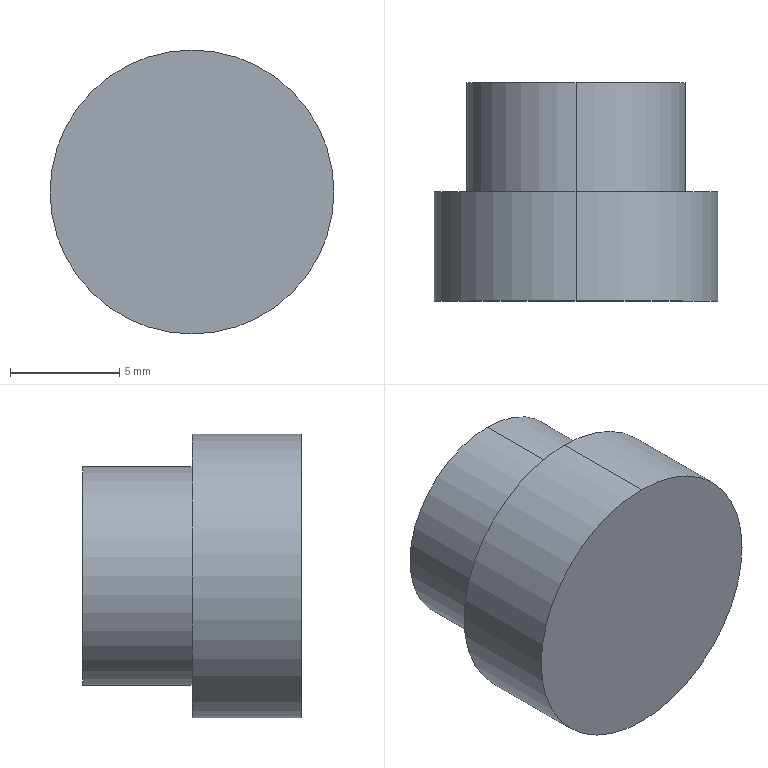Part | SolidWorks | features Revolution 1 | 1 solid | 10 faces | box 13 x 10 x 13 mm | volume 805.033 mm3 | cylinder 6 | plane 4 | commonest cylinder face diameters 8 x2 10 x2 13 x2
STEP:
#1=CARTESIAN_POINT('',(0.,10.,4.));
#2=VERTEX_POINT('',#1);
#3=CARTESIAN_POINT('',(0.,10.,-4.));
#4=VERTEX_POINT('',#3);
#5=CARTESIAN_POINT('',(0.,10.,0.));
#6=DIRECTION('',(0.,-1.,0.));
#7=DIRECTION('',(0.,0.,-1.));
#8=AXIS2_PLACEMENT_3D('',#5,#6,#7);
#9=CIRCLE('',#8,4.);
#10=EDGE_CURVE('',#2,#4,#9,.T.);
#11=ORIENTED_EDGE('',*,*,#10,.F.);
#12=CARTESIAN_POINT('',(0.,5.,4.));
#13=VERTEX_POINT('',#12);
#14=CARTESIAN_POINT('',(0.,0.,4.));
#15=DIRECTION('',(0.,-1.,0.));
#16=VECTOR('',#15,1000.);
#17=LINE('',#14,#16);
#18=EDGE_CURVE('',#2,#13,#17,.T.);
#19=ORIENTED_EDGE('',*,*,#18,.T.);
#20=CARTESIAN_POINT('',(0.,5.,-4.));
#21=VERTEX_POINT('',#20);
#22=CARTESIAN_POINT('',(0.,5.,0.));
#23=DIRECTION('',(0.,-1.,0.));
#24=DIRECTION('',(0.,0.,-1.));
#25=AXIS2_PLACEMENT_3D('',#22,#23,#24);
#26=CIRCLE('',#25,4.);
#27=EDGE_CURVE('',#13,#21,#26,.T.);
#28=ORIENTED_EDGE('',*,*,#27,.T.);
#29=CARTESIAN_POINT('',(0.,0.,-4.));
#30=DIRECTION('',(0.,-1.,0.));
#31=VECTOR('',#30,1000.);
#32=LINE('',#29,#31);
#33=EDGE_CURVE('',#4,#21,#32,.T.);
#34=ORIENTED_EDGE('',*,*,#33,.F.);
#35=EDGE_LOOP('',(#11,#19,#28,#34));
#36=FACE_OUTER_BOUND('',#35,.T.);
#37=CARTESIAN_POINT('',(0.,0.,0.));
#38=DIRECTION('',(0.,-1.,0.));
#39=DIRECTION('',(0.,0.,-1.));
#40=AXIS2_PLACEMENT_3D('',#37,#38,#39);
#41=CYLINDRICAL_SURFACE('',#40,4.);
#42=ADVANCED_FACE('',(#36),#41,.F.);
#43=CARTESIAN_POINT('',(0.,10.,-5.));
#44=VERTEX_POINT('',#43);
#45=CARTESIAN_POINT('',(0.,10.,5.));
#46=VERTEX_POINT('',#45);
#47=CARTESIAN_POINT('',(0.,10.,0.));
#48=DIRECTION('',(0.,-1.,0.));
#49=DIRECTION('',(0.,0.,-1.));
#50=AXIS2_PLACEMENT_3D('',#47,#48,#49);
#51=CIRCLE('',#50,5.);
#52=EDGE_CURVE('',#44,#46,#51,.T.);
#53=ORIENTED_EDGE('',*,*,#52,.T.);
#54=CARTESIAN_POINT('',(0.,5.,5.));
#55=VERTEX_POINT('',#54);
#56=CARTESIAN_POINT('',(0.,0.,5.));
#57=DIRECTION('',(0.,-1.,0.));
#58=VECTOR('',#57,1000.);
#59=LINE('',#56,#58);
#60=EDGE_CURVE('',#46,#55,#59,.T.);
#61=ORIENTED_EDGE('',*,*,#60,.T.);
#62=CARTESIAN_POINT('',(0.,5.,-5.));
#63=VERTEX_POINT('',#62);
#64=CARTESIAN_POINT('',(0.,5.,0.));
#65=DIRECTION('',(0.,-1.,0.));
#66=DIRECTION('',(0.,0.,-1.));
#67=AXIS2_PLACEMENT_3D('',#64,#65,#66);
#68=CIRCLE('',#67,5.);
#69=EDGE_CURVE('',#63,#55,#68,.T.);
#70=ORIENTED_EDGE('',*,*,#69,.F.);
#71=CARTESIAN_POINT('',(0.,0.,-5.));
#72=DIRECTION('',(0.,-1.,0.));
#73=VECTOR('',#72,1000.);
#74=LINE('',#71,#73);
#75=EDGE_CURVE('',#44,#63,#74,.T.);
#76=ORIENTED_EDGE('',*,*,#75,.F.);
#77=EDGE_LOOP('',(#53,#61,#70,#76));
#78=FACE_OUTER_BOUND('',#77,.T.);
#79=CARTESIAN_POINT('',(0.,0.,0.));
#80=DIRECTION('',(0.,-1.,0.));
#81=DIRECTION('',(0.,0.,-1.));
#82=AXIS2_PLACEMENT_3D('',#79,#80,#81);
#83=CYLINDRICAL_SURFACE('',#82,5.);
#84=ADVANCED_FACE('',(#78),#83,.T.);
#85=CARTESIAN_POINT('',(0.,5.,-6.5));
#86=VERTEX_POINT('',#85);
#87=CARTESIAN_POINT('',(0.,5.,6.5));
#88=VERTEX_POINT('',#87);
#89=CARTESIAN_POINT('',(0.,5.,0.));
#90=DIRECTION('',(0.,-1.,0.));
#91=DIRECTION('',(0.,0.,-1.));
#92=AXIS2_PLACEMENT_3D('',#89,#90,#91);
#93=CIRCLE('',#92,6.5);
#94=EDGE_CURVE('',#86,#88,#93,.T.);
#95=ORIENTED_EDGE('',*,*,#94,.T.);
#96=CARTESIAN_POINT('',(0.,0.,6.5));
#97=VERTEX_POINT('',#96);
#98=CARTESIAN_POINT('',(0.,0.,6.5));
#99=DIRECTION('',(0.,-1.,0.));
#100=VECTOR('',#99,1000.);
#101=LINE('',#98,#100);
#102=EDGE_CURVE('',#88,#97,#101,.T.);
#103=ORIENTED_EDGE('',*,*,#102,.T.);
#104=CARTESIAN_POINT('',(0.,0.,-6.5));
#105=VERTEX_POINT('',#104);
#106=CARTESIAN_POINT('',(0.,0.,0.));
#107=DIRECTION('',(0.,-1.,0.));
#108=DIRECTION('',(0.,0.,-1.));
#109=AXIS2_PLACEMENT_3D('',#106,#107,#108);
#110=CIRCLE('',#109,6.5);
#111=EDGE_CURVE('',#105,#97,#110,.T.);
#112=ORIENTED_EDGE('',*,*,#111,.F.);
#113=CARTESIAN_POINT('',(0.,0.,-6.5));
#114=DIRECTION('',(0.,-1.,0.));
#115=VECTOR('',#114,1000.);
#116=LINE('',#113,#115);
#117=EDGE_CURVE('',#86,#105,#116,.T.);
#118=ORIENTED_EDGE('',*,*,#117,.F.);
#119=EDGE_LOOP('',(#95,#103,#112,#118));
#120=FACE_OUTER_BOUND('',#119,.T.);
#121=CARTESIAN_POINT('',(0.,0.,0.));
#122=DIRECTION('',(0.,-1.,0.));
#123=DIRECTION('',(0.,0.,-1.));
#124=AXIS2_PLACEMENT_3D('',#121,#122,#123);
#125=CYLINDRICAL_SURFACE('',#124,6.5);
#126=ADVANCED_FACE('',(#120),#125,.T.);
#127=ORIENTED_EDGE('',*,*,#111,.T.);
#128=CARTESIAN_POINT('',(0.,0.,0.));
#129=DIRECTION('',(0.,-1.,0.));
#130=DIRECTION('',(0.,0.,-1.));
#131=AXIS2_PLACEMENT_3D('',#128,#129,#130);
#132=CIRCLE('',#131,6.5);
#133=EDGE_CURVE('',#97,#105,#132,.T.);
#134=ORIENTED_EDGE('',*,*,#133,.T.);
#135=EDGE_LOOP('',(#127,#134));
#136=FACE_OUTER_BOUND('',#135,.T.);
#137=CARTESIAN_POINT('',(0.,0.,0.));
#138=DIRECTION('',(0.,-1.,0.));
#139=DIRECTION('',(0.,0.,-1.));
#140=AXIS2_PLACEMENT_3D('',#137,#138,#139);
#141=PLANE('',#140);
#142=ADVANCED_FACE('',(#136),#141,.T.);
#143=ORIENTED_EDGE('',*,*,#102,.F.);
#144=CARTESIAN_POINT('',(0.,5.,0.));
#145=DIRECTION('',(0.,-1.,0.));
#146=DIRECTION('',(0.,0.,-1.));
#147=AXIS2_PLACEMENT_3D('',#144,#145,#146);
#148=CIRCLE('',#147,6.5);
#149=EDGE_CURVE('',#88,#86,#148,.T.);
#150=ORIENTED_EDGE('',*,*,#149,.T.);
#151=ORIENTED_EDGE('',*,*,#117,.T.);
#152=ORIENTED_EDGE('',*,*,#133,.F.);
#153=EDGE_LOOP('',(#143,#150,#151,#152));
#154=FACE_OUTER_BOUND('',#153,.T.);
#155=CARTESIAN_POINT('',(0.,0.,0.));
#156=DIRECTION('',(0.,-1.,0.));
#157=DIRECTION('',(0.,0.,-1.));
#158=AXIS2_PLACEMENT_3D('',#155,#156,#157);
#159=CYLINDRICAL_SURFACE('',#158,6.5);
#160=ADVANCED_FACE('',(#154),#159,.T.);
#161=ORIENTED_EDGE('',*,*,#69,.T.);
#162=CARTESIAN_POINT('',(0.,5.,0.));
#163=DIRECTION('',(0.,-1.,0.));
#164=DIRECTION('',(0.,0.,-1.));
#165=AXIS2_PLACEMENT_3D('',#162,#163,#164);
#166=CIRCLE('',#165,5.);
#167=EDGE_CURVE('',#55,#63,#166,.T.);
#168=ORIENTED_EDGE('',*,*,#167,.T.);
#169=EDGE_LOOP('',(#161,#168));
#170=FACE_BOUND('',#169,.T.);
#171=ORIENTED_EDGE('',*,*,#94,.F.);
#172=ORIENTED_EDGE('',*,*,#149,.F.);
#173=EDGE_LOOP('',(#171,#172));
#174=FACE_OUTER_BOUND('',#173,.T.);
#175=CARTESIAN_POINT('',(6.5,5.,0.));
#176=DIRECTION('',(0.,1.,0.));
#177=DIRECTION('',(0.,0.,1.));
#178=AXIS2_PLACEMENT_3D('',#175,#176,#177);
#179=PLANE('',#178);
#180=ADVANCED_FACE('',(#170,#174),#179,.T.);
#181=ORIENTED_EDGE('',*,*,#60,.F.);
#182=CARTESIAN_POINT('',(0.,10.,0.));
#183=DIRECTION('',(0.,-1.,0.));
#184=DIRECTION('',(0.,0.,-1.));
#185=AXIS2_PLACEMENT_3D('',#182,#183,#184);
#186=CIRCLE('',#185,5.);
#187=EDGE_CURVE('',#46,#44,#186,.T.);
#188=ORIENTED_EDGE('',*,*,#187,.T.);
#189=ORIENTED_EDGE('',*,*,#75,.T.);
#190=ORIENTED_EDGE('',*,*,#167,.F.);
#191=EDGE_LOOP('',(#181,#188,#189,#190));
#192=FACE_OUTER_BOUND('',#191,.T.);
#193=CARTESIAN_POINT('',(0.,0.,0.));
#194=DIRECTION('',(0.,-1.,0.));
#195=DIRECTION('',(0.,0.,-1.));
#196=AXIS2_PLACEMENT_3D('',#193,#194,#195);
#197=CYLINDRICAL_SURFACE('',#196,5.);
#198=ADVANCED_FACE('',(#192),#197,.T.);
#199=CARTESIAN_POINT('',(0.,10.,0.));
#200=DIRECTION('',(0.,-1.,0.));
#201=DIRECTION('',(0.,0.,-1.));
#202=AXIS2_PLACEMENT_3D('',#199,#200,#201);
#203=CIRCLE('',#202,4.);
#204=EDGE_CURVE('',#4,#2,#203,.T.);
#205=ORIENTED_EDGE('',*,*,#204,.T.);
#206=ORIENTED_EDGE('',*,*,#10,.T.);
#207=EDGE_LOOP('',(#205,#206));
#208=FACE_BOUND('',#207,.T.);
#209=ORIENTED_EDGE('',*,*,#52,.F.);
#210=ORIENTED_EDGE('',*,*,#187,.F.);
#211=EDGE_LOOP('',(#209,#210));
#212=FACE_OUTER_BOUND('',#211,.T.);
#213=CARTESIAN_POINT('',(5.,10.,0.));
#214=DIRECTION('',(0.,1.,0.));
#215=DIRECTION('',(0.,0.,1.));
#216=AXIS2_PLACEMENT_3D('',#213,#214,#215);
#217=PLANE('',#216);
#218=ADVANCED_FACE('',(#208,#212),#217,.T.);
#219=ORIENTED_EDGE('',*,*,#18,.F.);
#220=ORIENTED_EDGE('',*,*,#204,.F.);
#221=ORIENTED_EDGE('',*,*,#33,.T.);
#222=CARTESIAN_POINT('',(0.,5.,0.));
#223=DIRECTION('',(0.,-1.,0.));
#224=DIRECTION('',(0.,0.,-1.));
#225=AXIS2_PLACEMENT_3D('',#222,#223,#224);
#226=CIRCLE('',#225,4.);
#227=EDGE_CURVE('',#21,#13,#226,.T.);
#228=ORIENTED_EDGE('',*,*,#227,.T.);
#229=EDGE_LOOP('',(#219,#220,#221,#228));
#230=FACE_OUTER_BOUND('',#229,.T.);
#231=CARTESIAN_POINT('',(0.,0.,0.));
#232=DIRECTION('',(0.,-1.,0.));
#233=DIRECTION('',(0.,0.,-1.));
#234=AXIS2_PLACEMENT_3D('',#231,#232,#233);
#235=CYLINDRICAL_SURFACE('',#234,4.);
#236=ADVANCED_FACE('',(#230),#235,.F.);
#237=ORIENTED_EDGE('',*,*,#227,.F.);
#238=ORIENTED_EDGE('',*,*,#27,.F.);
#239=EDGE_LOOP('',(#237,#238));
#240=FACE_OUTER_BOUND('',#239,.T.);
#241=CARTESIAN_POINT('',(4.,5.,0.));
#242=DIRECTION('',(0.,1.,0.));
#243=DIRECTION('',(0.,0.,1.));
#244=AXIS2_PLACEMENT_3D('',#241,#242,#243);
#245=PLANE('',#244);
#246=ADVANCED_FACE('',(#240),#245,.T.);
#247=CLOSED_SHELL('',(#42,#84,#126,#142,#160,#180,#198,#218,#236,#246));
#248=MANIFOLD_SOLID_BREP('',#247);
#249=CARTESIAN_POINT('',(0.,0.,0.));
#250=DIRECTION('',(0.,0.,1.));
#251=DIRECTION('',(1.,0.,0.));
#252=AXIS2_PLACEMENT_3D('',#249,#250,#251);
#253=(LENGTH_UNIT()NAMED_UNIT(*)SI_UNIT(.MILLI.,.METRE.));
#254=UNCERTAINTY_MEASURE_WITH_UNIT(LENGTH_MEASURE(0.00001),#253,'','');
#255=(NAMED_UNIT(*)PLANE_ANGLE_UNIT()SI_UNIT($,.RADIAN.));
#256=(NAMED_UNIT(*)SI_UNIT($,.STERADIAN.)SOLID_ANGLE_UNIT());
#257=(GEOMETRIC_REPRESENTATION_CONTEXT(3)GLOBAL_UNCERTAINTY_ASSIGNED_CONTEXT((#254))GLOBAL_UNIT_ASSIGNED_CONTEXT((#253,#255,#256))REPRESENTATION_CONTEXT('',''));
#258=ADVANCED_BREP_SHAPE_REPRESENTATION('',(#248,#252),#257);